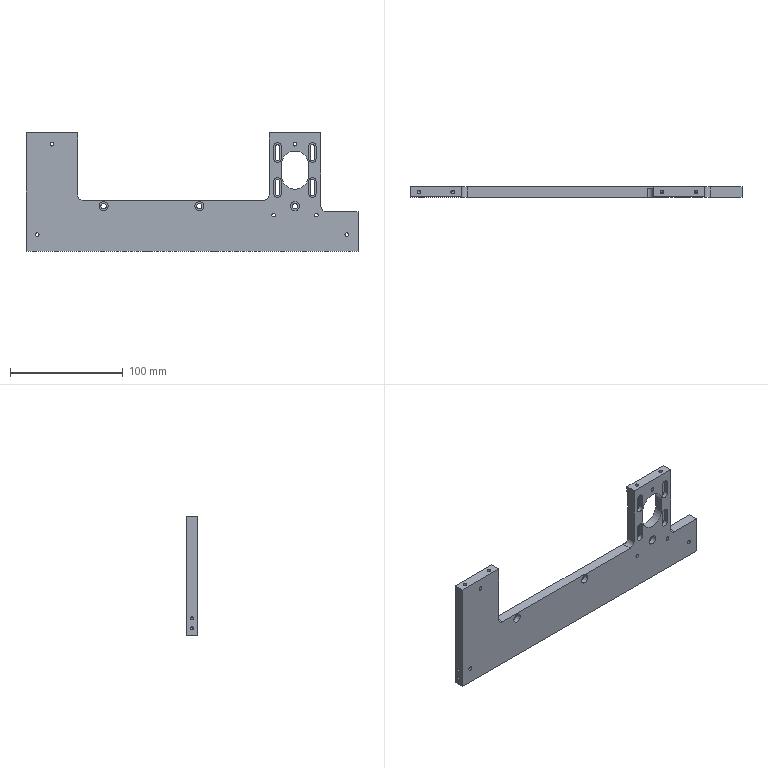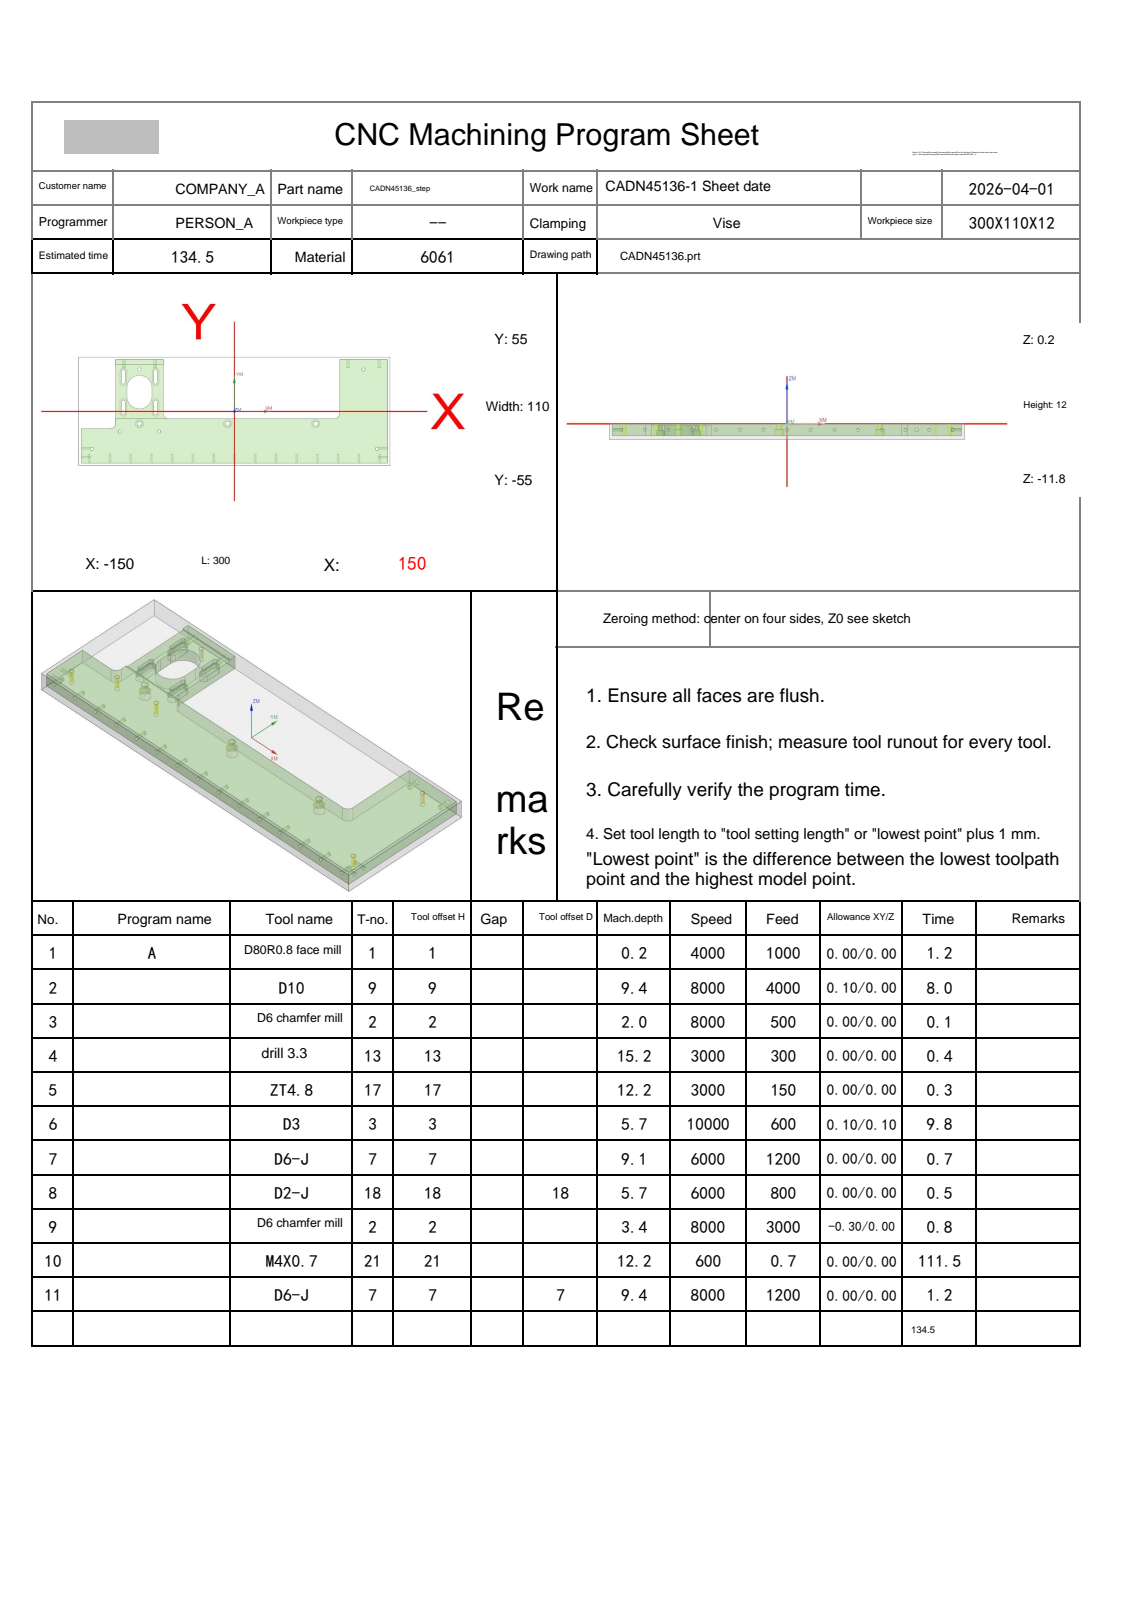NC program | NX | posted by the shop | part box 295 x 9 x 105 mm
Lines 1 to 39 of 7463:
%
O0001
(Machine time: 239.39 MIN)
(===Total Tool:9===)
(T1=D80R0.8 face mill D=80.  R=0.8  D-  H01 Z=0.    )
(T9=D10     D=10.  R=0.   D-  H09 Z=-9.2  )
(T2=D6 chamfer mill   D=6.   R=0.   D-  H02 Z=-3.2  )
(T13=drill 3.3  D=3.3  DR_a=118 D-  H13 Z=-14.99)
(T17=ZT4.8  D=4.8  DR_a=118 D-  H17 Z=-12.  )
(T3=D3      D=3.   R=0.   D-  H03 Z=-5.5  )
(T7=D6-J    D=6.   R=0.   D7  H07 Z=-9.2  )
(T18=D2-J   D=2.   R=0.   D18 H18 Z=-5.5  )
(T21=M4X0.7 D=3.3  DR_a=180 D-  H21 Z=-12.  )
G80 G90 G17 G49 G40
G91 G28 Z0
M01
N1 T01 M06
(D80R0.8 face mill  D=80. R=0.8 H=01 ce=0.00 di=0.00)
G00 G90 G54 X-192.5 Y46.25 M03 S4000
G43 H01 Z20.
M08
Z2.
G01 Z0.0 F1000.
X-187.5
X187.5
Y0.0
X-187.5
Y-46.25
X187.5
X192.5
Z2.
G00 Z20.
G91 G28 Z0.0
M05
M09
G91 G28 Z0.0
M01